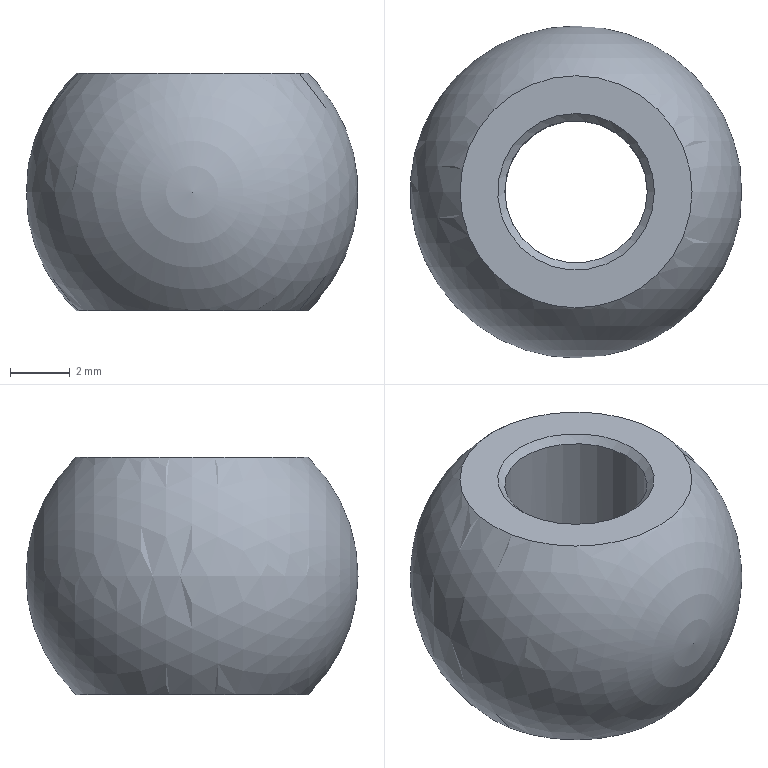Part | NX | features 2458K311 2 | 1 solid | 6 faces | box 11.1 x 11.1 x 7.938 mm | volume 494.869 mm3 | plane 2 | cone 2 | sphere 1 | cylinder 1 | commonest cylinder face diameters 4.763 x1
STEP:
#1=CARTESIAN_POINT('',(0.,10.408,-3.969));
#2=VERTEX_POINT('',#1);
#3=CARTESIAN_POINT('',(0.,14.287,-3.969));
#4=DIRECTION('',(0.,0.,1.));
#5=DIRECTION('',(0.,-1.,0.));
#6=AXIS2_PLACEMENT_3D('',#3,#4,#5);
#7=CIRCLE('',#6,3.879);
#8=EDGE_CURVE('',#2,#2,#7,.F.);
#9=ORIENTED_EDGE('',*,*,#8,.F.);
#10=EDGE_LOOP('',(#9));
#11=FACE_BOUND('',#10,.T.);
#12=CARTESIAN_POINT('',(0.,18.167,3.969));
#13=VERTEX_POINT('',#12);
#14=CARTESIAN_POINT('',(0.,14.287,3.969));
#15=DIRECTION('',(0.,0.,-1.));
#16=DIRECTION('',(0.,1.,0.));
#17=AXIS2_PLACEMENT_3D('',#14,#15,#16);
#18=CIRCLE('',#17,3.879);
#19=EDGE_CURVE('',#13,#13,#18,.F.);
#20=ORIENTED_EDGE('',*,*,#19,.F.);
#21=EDGE_LOOP('',(#20));
#22=FACE_BOUND('',#21,.T.);
#23=CARTESIAN_POINT('',(0.,14.287,0.));
#24=DIRECTION('',(0.,-1.,0.));
#25=DIRECTION('',(1.,0.,0.));
#26=AXIS2_PLACEMENT_3D('',#23,#24,#25);
#27=SPHERICAL_SURFACE('',#26,5.55);
#28=ADVANCED_FACE('',(#11,#22),#27,.T.);
#29=CARTESIAN_POINT('',(0.,16.907,3.969));
#30=VERTEX_POINT('',#29);
#31=CARTESIAN_POINT('',(0.,14.287,3.969));
#32=DIRECTION('',(0.,0.,-1.));
#33=DIRECTION('',(0.,1.,0.));
#34=AXIS2_PLACEMENT_3D('',#31,#32,#33);
#35=CIRCLE('',#34,2.619);
#36=EDGE_CURVE('',#30,#30,#35,.T.);
#37=ORIENTED_EDGE('',*,*,#36,.T.);
#38=EDGE_LOOP('',(#37));
#39=FACE_BOUND('',#38,.T.);
#40=ORIENTED_EDGE('',*,*,#19,.T.);
#41=EDGE_LOOP('',(#40));
#42=FACE_BOUND('',#41,.T.);
#43=CARTESIAN_POINT('',(-7.938,22.225,3.969));
#44=DIRECTION('',(0.,0.,-1.));
#45=DIRECTION('',(0.,1.,0.));
#46=AXIS2_PLACEMENT_3D('',#43,#44,#45);
#47=PLANE('',#46);
#48=ADVANCED_FACE('',(#39,#42),#47,.F.);
#49=CARTESIAN_POINT('',(0.,11.668,-3.969));
#50=VERTEX_POINT('',#49);
#51=CARTESIAN_POINT('',(0.,14.287,-3.969));
#52=DIRECTION('',(0.,0.,1.));
#53=DIRECTION('',(0.,-1.,0.));
#54=AXIS2_PLACEMENT_3D('',#51,#52,#53);
#55=CIRCLE('',#54,2.619);
#56=EDGE_CURVE('',#50,#50,#55,.T.);
#57=ORIENTED_EDGE('',*,*,#56,.T.);
#58=EDGE_LOOP('',(#57));
#59=FACE_BOUND('',#58,.T.);
#60=ORIENTED_EDGE('',*,*,#8,.T.);
#61=EDGE_LOOP('',(#60));
#62=FACE_BOUND('',#61,.T.);
#63=CARTESIAN_POINT('',(-7.938,22.225,-3.969));
#64=DIRECTION('',(0.,0.,1.));
#65=DIRECTION('',(0.,-1.,0.));
#66=AXIS2_PLACEMENT_3D('',#63,#64,#65);
#67=PLANE('',#66);
#68=ADVANCED_FACE('',(#59,#62),#67,.F.);
#69=CARTESIAN_POINT('',(2.381,14.287,-3.731));
#70=VERTEX_POINT('',#69);
#71=CARTESIAN_POINT('',(0.,14.287,-3.731));
#72=DIRECTION('',(0.,0.,1.));
#73=DIRECTION('',(1.,0.,0.));
#74=AXIS2_PLACEMENT_3D('',#71,#72,#73);
#75=CIRCLE('',#74,2.381);
#76=EDGE_CURVE('',#70,#70,#75,.F.);
#77=ORIENTED_EDGE('',*,*,#76,.T.);
#78=EDGE_LOOP('',(#77));
#79=FACE_BOUND('',#78,.T.);
#80=CARTESIAN_POINT('',(-2.381,14.287,3.731));
#81=VERTEX_POINT('',#80);
#82=CARTESIAN_POINT('',(0.,14.287,3.731));
#83=DIRECTION('',(0.,0.,-1.));
#84=DIRECTION('',(-1.,0.,0.));
#85=AXIS2_PLACEMENT_3D('',#82,#83,#84);
#86=CIRCLE('',#85,2.381);
#87=EDGE_CURVE('',#81,#81,#86,.F.);
#88=ORIENTED_EDGE('',*,*,#87,.T.);
#89=EDGE_LOOP('',(#88));
#90=FACE_BOUND('',#89,.T.);
#91=CARTESIAN_POINT('',(0.,14.287,-4.706));
#92=DIRECTION('',(0.,0.,1.));
#93=DIRECTION('',(1.,0.,0.));
#94=AXIS2_PLACEMENT_3D('',#91,#92,#93);
#95=CYLINDRICAL_SURFACE('',#94,2.381);
#96=ADVANCED_FACE('',(#79,#90),#95,.F.);
#97=ORIENTED_EDGE('',*,*,#76,.F.);
#98=EDGE_LOOP('',(#97));
#99=FACE_BOUND('',#98,.T.);
#100=ORIENTED_EDGE('',*,*,#56,.F.);
#101=EDGE_LOOP('',(#100));
#102=FACE_BOUND('',#101,.T.);
#103=CARTESIAN_POINT('',(0.,14.287,-3.969));
#104=DIRECTION('',(0.,0.,-1.));
#105=DIRECTION('',(-1.,0.,0.));
#106=AXIS2_PLACEMENT_3D('',#103,#104,#105);
#107=CONICAL_SURFACE('',#106,2.619,0.7854);
#108=ADVANCED_FACE('',(#99,#102),#107,.F.);
#109=ORIENTED_EDGE('',*,*,#87,.F.);
#110=EDGE_LOOP('',(#109));
#111=FACE_BOUND('',#110,.T.);
#112=ORIENTED_EDGE('',*,*,#36,.F.);
#113=EDGE_LOOP('',(#112));
#114=FACE_BOUND('',#113,.T.);
#115=CARTESIAN_POINT('',(0.,14.287,3.969));
#116=DIRECTION('',(0.,0.,1.));
#117=DIRECTION('',(1.,0.,0.));
#118=AXIS2_PLACEMENT_3D('',#115,#116,#117);
#119=CONICAL_SURFACE('',#118,2.619,0.7854);
#120=ADVANCED_FACE('',(#111,#114),#119,.F.);
#121=CLOSED_SHELL('',(#28,#48,#68,#96,#108,#120));
#122=MANIFOLD_SOLID_BREP('',#121);
#123=(LENGTH_UNIT()NAMED_UNIT(*)SI_UNIT(.MILLI.,.METRE.));
#124=UNCERTAINTY_MEASURE_WITH_UNIT(LENGTH_MEASURE(0.00001),#123,'','');
#125=(NAMED_UNIT(*)PLANE_ANGLE_UNIT()SI_UNIT($,.RADIAN.));
#126=(NAMED_UNIT(*)SI_UNIT($,.STERADIAN.)SOLID_ANGLE_UNIT());
#127=(GEOMETRIC_REPRESENTATION_CONTEXT(3)GLOBAL_UNCERTAINTY_ASSIGNED_CONTEXT((#124))GLOBAL_UNIT_ASSIGNED_CONTEXT((#123,#125,#126))REPRESENTATION_CONTEXT('',''));
#128=ADVANCED_BREP_SHAPE_REPRESENTATION('',(#122),#127);